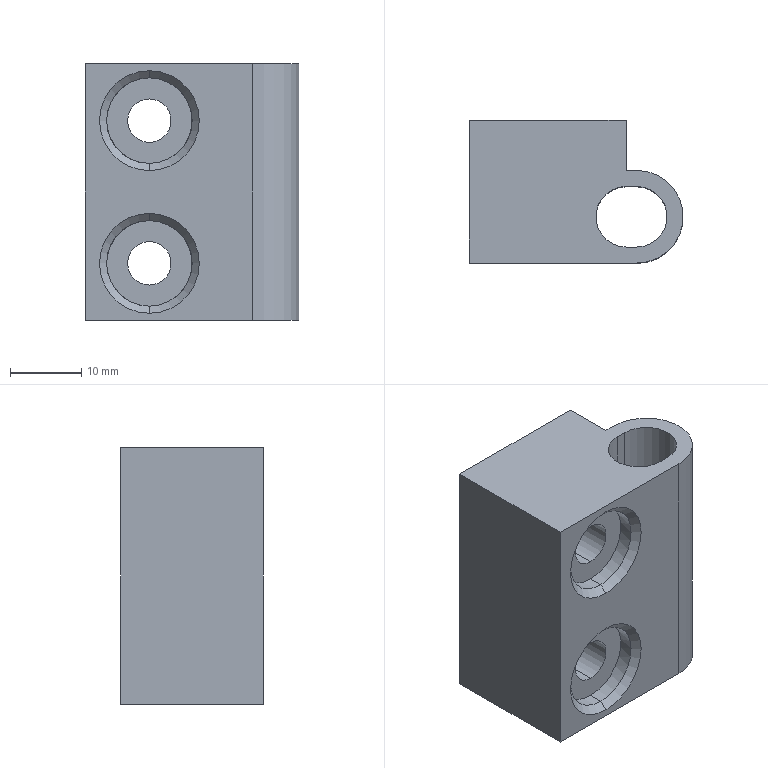Part | STEP file | _X2_751F4E45_X0_RG004-3_X2_5BFC | 1 solid | 26 faces | box 30 x 20 x 36 mm | volume 14717 mm3 | plane 11 | cylinder 11 | cone 4 | commonest cylinder face diameters 6.1 x4 12 x4 8.5 x2 13 x1